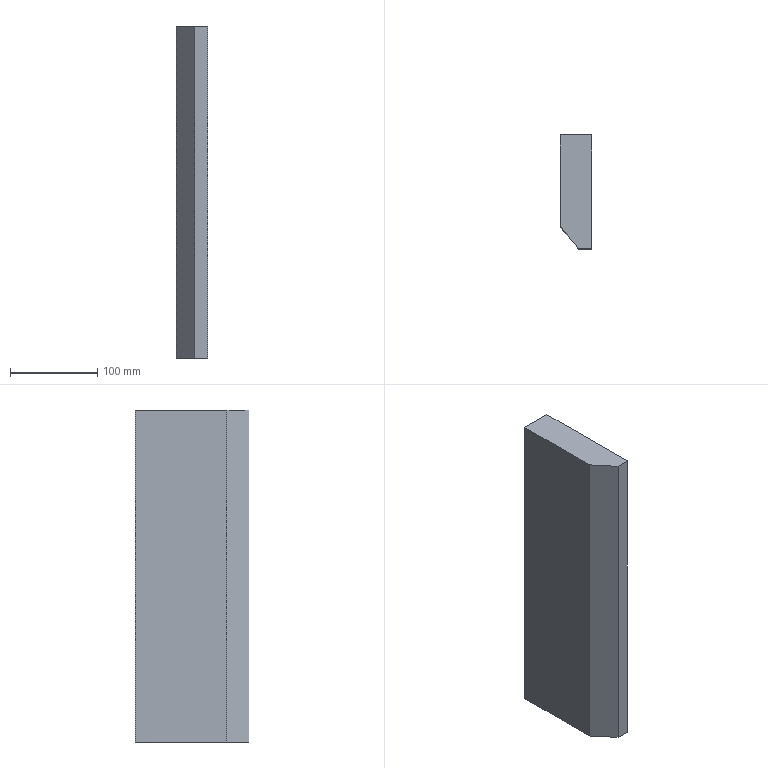Part | SolidWorks | features Extrusion 1 | 1 solid | 7 faces | box 36 x 130 x 380 mm | volume 1678543 mm3 | plane 7
STEP:
#1=CARTESIAN_POINT('',(-15.,0.,-190.));
#2=VERTEX_POINT('',#1);
#3=CARTESIAN_POINT('',(0.,0.,-190.));
#4=VERTEX_POINT('',#3);
#5=CARTESIAN_POINT('',(-15.,0.,-190.));
#6=DIRECTION('',(1.,0.,0.));
#7=VECTOR('',#6,1000.);
#8=LINE('',#5,#7);
#9=EDGE_CURVE('',#2,#4,#8,.T.);
#10=ORIENTED_EDGE('',*,*,#9,.T.);
#11=CARTESIAN_POINT('',(0.,0.,190.));
#12=VERTEX_POINT('',#11);
#13=CARTESIAN_POINT('',(0.,0.,190.));
#14=DIRECTION('',(0.,0.,-1.));
#15=VECTOR('',#14,1000.);
#16=LINE('',#13,#15);
#17=EDGE_CURVE('',#12,#4,#16,.T.);
#18=ORIENTED_EDGE('',*,*,#17,.F.);
#19=CARTESIAN_POINT('',(-15.,0.,190.));
#20=VERTEX_POINT('',#19);
#21=CARTESIAN_POINT('',(-15.,0.,190.));
#22=DIRECTION('',(1.,0.,0.));
#23=VECTOR('',#22,1000.);
#24=LINE('',#21,#23);
#25=EDGE_CURVE('',#20,#12,#24,.T.);
#26=ORIENTED_EDGE('',*,*,#25,.F.);
#27=CARTESIAN_POINT('',(-15.,0.,190.));
#28=DIRECTION('',(0.,0.,-1.));
#29=VECTOR('',#28,1000.);
#30=LINE('',#27,#29);
#31=EDGE_CURVE('',#20,#2,#30,.T.);
#32=ORIENTED_EDGE('',*,*,#31,.T.);
#33=EDGE_LOOP('',(#10,#18,#26,#32));
#34=FACE_OUTER_BOUND('',#33,.T.);
#35=CARTESIAN_POINT('',(-15.,0.,190.));
#36=DIRECTION('',(0.,1.,0.));
#37=DIRECTION('',(0.,0.,1.));
#38=AXIS2_PLACEMENT_3D('',#35,#36,#37);
#39=PLANE('',#38);
#40=ADVANCED_FACE('',(#34),#39,.F.);
#41=CARTESIAN_POINT('',(0.,130.,-190.));
#42=VERTEX_POINT('',#41);
#43=CARTESIAN_POINT('',(0.,0.,-190.));
#44=DIRECTION('',(0.,1.,0.));
#45=VECTOR('',#44,1000.);
#46=LINE('',#43,#45);
#47=EDGE_CURVE('',#4,#42,#46,.T.);
#48=ORIENTED_EDGE('',*,*,#47,.T.);
#49=CARTESIAN_POINT('',(0.,130.,190.));
#50=VERTEX_POINT('',#49);
#51=CARTESIAN_POINT('',(0.,130.,190.));
#52=DIRECTION('',(0.,0.,-1.));
#53=VECTOR('',#52,1000.);
#54=LINE('',#51,#53);
#55=EDGE_CURVE('',#50,#42,#54,.T.);
#56=ORIENTED_EDGE('',*,*,#55,.F.);
#57=CARTESIAN_POINT('',(0.,0.,190.));
#58=DIRECTION('',(0.,1.,0.));
#59=VECTOR('',#58,1000.);
#60=LINE('',#57,#59);
#61=EDGE_CURVE('',#12,#50,#60,.T.);
#62=ORIENTED_EDGE('',*,*,#61,.F.);
#63=ORIENTED_EDGE('',*,*,#17,.T.);
#64=EDGE_LOOP('',(#48,#56,#62,#63));
#65=FACE_OUTER_BOUND('',#64,.T.);
#66=CARTESIAN_POINT('',(0.,0.,190.));
#67=DIRECTION('',(-1.,0.,0.));
#68=DIRECTION('',(0.,0.,1.));
#69=AXIS2_PLACEMENT_3D('',#66,#67,#68);
#70=PLANE('',#69);
#71=ADVANCED_FACE('',(#65),#70,.F.);
#72=CARTESIAN_POINT('',(-36.,130.,-190.));
#73=VERTEX_POINT('',#72);
#74=CARTESIAN_POINT('',(0.,130.,-190.));
#75=DIRECTION('',(-1.,0.,0.));
#76=VECTOR('',#75,1000.);
#77=LINE('',#74,#76);
#78=EDGE_CURVE('',#42,#73,#77,.T.);
#79=ORIENTED_EDGE('',*,*,#78,.T.);
#80=CARTESIAN_POINT('',(-36.,130.,190.));
#81=VERTEX_POINT('',#80);
#82=CARTESIAN_POINT('',(-36.,130.,190.));
#83=DIRECTION('',(0.,0.,-1.));
#84=VECTOR('',#83,1000.);
#85=LINE('',#82,#84);
#86=EDGE_CURVE('',#81,#73,#85,.T.);
#87=ORIENTED_EDGE('',*,*,#86,.F.);
#88=CARTESIAN_POINT('',(0.,130.,190.));
#89=DIRECTION('',(-1.,0.,0.));
#90=VECTOR('',#89,1000.);
#91=LINE('',#88,#90);
#92=EDGE_CURVE('',#50,#81,#91,.T.);
#93=ORIENTED_EDGE('',*,*,#92,.F.);
#94=ORIENTED_EDGE('',*,*,#55,.T.);
#95=EDGE_LOOP('',(#79,#87,#93,#94));
#96=FACE_OUTER_BOUND('',#95,.T.);
#97=CARTESIAN_POINT('',(0.,130.,190.));
#98=DIRECTION('',(0.,-1.,0.));
#99=DIRECTION('',(0.,0.,-1.));
#100=AXIS2_PLACEMENT_3D('',#97,#98,#99);
#101=PLANE('',#100);
#102=ADVANCED_FACE('',(#96),#101,.F.);
#103=CARTESIAN_POINT('',(-36.,25.027,-190.));
#104=VERTEX_POINT('',#103);
#105=CARTESIAN_POINT('',(-36.,130.,-190.));
#106=DIRECTION('',(0.,-1.,0.));
#107=VECTOR('',#106,1000.);
#108=LINE('',#105,#107);
#109=EDGE_CURVE('',#73,#104,#108,.T.);
#110=ORIENTED_EDGE('',*,*,#109,.T.);
#111=CARTESIAN_POINT('',(-36.,25.027,190.));
#112=VERTEX_POINT('',#111);
#113=CARTESIAN_POINT('',(-36.,25.027,190.));
#114=DIRECTION('',(0.,0.,-1.));
#115=VECTOR('',#114,1000.);
#116=LINE('',#113,#115);
#117=EDGE_CURVE('',#112,#104,#116,.T.);
#118=ORIENTED_EDGE('',*,*,#117,.F.);
#119=CARTESIAN_POINT('',(-36.,130.,190.));
#120=DIRECTION('',(0.,-1.,0.));
#121=VECTOR('',#120,1000.);
#122=LINE('',#119,#121);
#123=EDGE_CURVE('',#81,#112,#122,.T.);
#124=ORIENTED_EDGE('',*,*,#123,.F.);
#125=ORIENTED_EDGE('',*,*,#86,.T.);
#126=EDGE_LOOP('',(#110,#118,#124,#125));
#127=FACE_OUTER_BOUND('',#126,.T.);
#128=CARTESIAN_POINT('',(-36.,130.,190.));
#129=DIRECTION('',(1.,0.,0.));
#130=DIRECTION('',(0.,1.,0.));
#131=AXIS2_PLACEMENT_3D('',#128,#129,#130);
#132=PLANE('',#131);
#133=ADVANCED_FACE('',(#127),#132,.F.);
#134=CARTESIAN_POINT('',(-36.,25.027,-190.));
#135=DIRECTION('',(0.6428,-0.766,0.));
#136=VECTOR('',#135,1000.);
#137=LINE('',#134,#136);
#138=EDGE_CURVE('',#104,#2,#137,.T.);
#139=ORIENTED_EDGE('',*,*,#138,.T.);
#140=ORIENTED_EDGE('',*,*,#31,.F.);
#141=CARTESIAN_POINT('',(-36.,25.027,190.));
#142=DIRECTION('',(0.6428,-0.766,0.));
#143=VECTOR('',#142,1000.);
#144=LINE('',#141,#143);
#145=EDGE_CURVE('',#112,#20,#144,.T.);
#146=ORIENTED_EDGE('',*,*,#145,.F.);
#147=ORIENTED_EDGE('',*,*,#117,.T.);
#148=EDGE_LOOP('',(#139,#140,#146,#147));
#149=FACE_OUTER_BOUND('',#148,.T.);
#150=CARTESIAN_POINT('',(-36.,25.027,190.));
#151=DIRECTION('',(0.766,0.6428,0.));
#152=DIRECTION('',(-0.6428,0.766,0.));
#153=AXIS2_PLACEMENT_3D('',#150,#151,#152);
#154=PLANE('',#153);
#155=ADVANCED_FACE('',(#149),#154,.F.);
#156=ORIENTED_EDGE('',*,*,#25,.T.);
#157=ORIENTED_EDGE('',*,*,#61,.T.);
#158=ORIENTED_EDGE('',*,*,#92,.T.);
#159=ORIENTED_EDGE('',*,*,#123,.T.);
#160=ORIENTED_EDGE('',*,*,#145,.T.);
#161=EDGE_LOOP('',(#156,#157,#158,#159,#160));
#162=FACE_OUTER_BOUND('',#161,.T.);
#163=CARTESIAN_POINT('',(0.,0.,190.));
#164=DIRECTION('',(0.,0.,1.));
#165=DIRECTION('',(1.,0.,0.));
#166=AXIS2_PLACEMENT_3D('',#163,#164,#165);
#167=PLANE('',#166);
#168=ADVANCED_FACE('',(#162),#167,.T.);
#169=ORIENTED_EDGE('',*,*,#9,.F.);
#170=ORIENTED_EDGE('',*,*,#138,.F.);
#171=ORIENTED_EDGE('',*,*,#109,.F.);
#172=ORIENTED_EDGE('',*,*,#78,.F.);
#173=ORIENTED_EDGE('',*,*,#47,.F.);
#174=EDGE_LOOP('',(#169,#170,#171,#172,#173));
#175=FACE_OUTER_BOUND('',#174,.T.);
#176=CARTESIAN_POINT('',(0.,0.,-190.));
#177=DIRECTION('',(0.,0.,1.));
#178=DIRECTION('',(1.,0.,0.));
#179=AXIS2_PLACEMENT_3D('',#176,#177,#178);
#180=PLANE('',#179);
#181=ADVANCED_FACE('',(#175),#180,.F.);
#182=CLOSED_SHELL('',(#40,#71,#102,#133,#155,#168,#181));
#183=MANIFOLD_SOLID_BREP('',#182);
#184=CARTESIAN_POINT('',(0.,0.,0.));
#185=DIRECTION('',(0.,0.,1.));
#186=DIRECTION('',(1.,0.,0.));
#187=AXIS2_PLACEMENT_3D('',#184,#185,#186);
#188=(LENGTH_UNIT()NAMED_UNIT(*)SI_UNIT(.MILLI.,.METRE.));
#189=UNCERTAINTY_MEASURE_WITH_UNIT(LENGTH_MEASURE(0.00001),#188,'','');
#190=(NAMED_UNIT(*)PLANE_ANGLE_UNIT()SI_UNIT($,.RADIAN.));
#191=(NAMED_UNIT(*)SI_UNIT($,.STERADIAN.)SOLID_ANGLE_UNIT());
#192=(GEOMETRIC_REPRESENTATION_CONTEXT(3)GLOBAL_UNCERTAINTY_ASSIGNED_CONTEXT((#189))GLOBAL_UNIT_ASSIGNED_CONTEXT((#188,#190,#191))REPRESENTATION_CONTEXT('',''));
#193=ADVANCED_BREP_SHAPE_REPRESENTATION('',(#183,#187),#192);